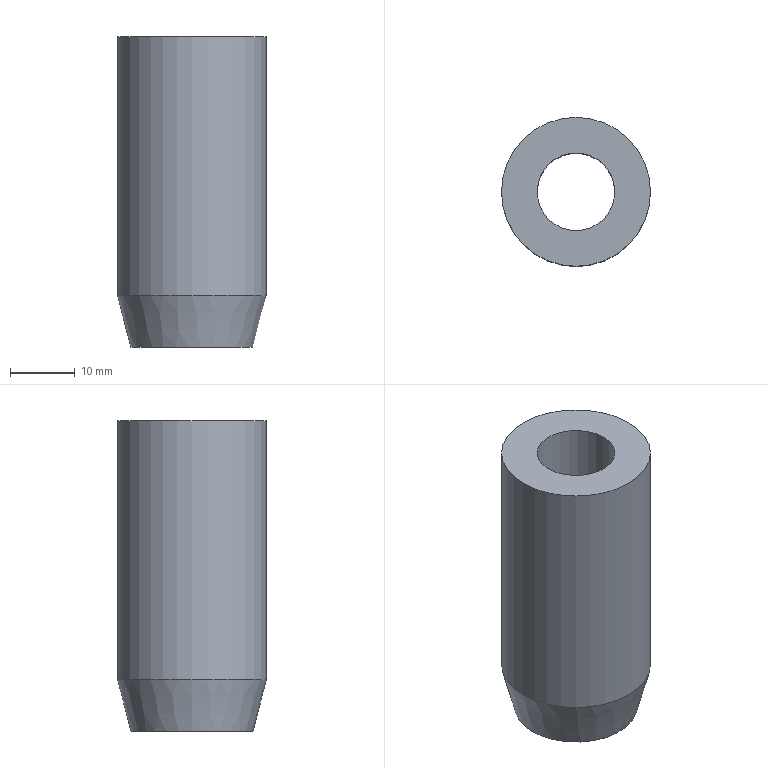Part | NX | features solid 2 | 1 solid | 5 faces | box 23 x 23 x 48 mm | volume 13952 mm3 | plane 2 | cylinder 2 | cone 1 | commonest cylinder face diameters 12 x1 23 x1
STEP:
#1=CARTESIAN_POINT('',(123.5,-300.,315.));
#2=VERTEX_POINT('',#1);
#3=CARTESIAN_POINT('',(135.,-300.,315.));
#4=DIRECTION('',(0.,0.,-1.));
#5=DIRECTION('',(-1.,0.,0.));
#6=AXIS2_PLACEMENT_3D('',#3,#4,#5);
#7=CIRCLE('',#6,11.5);
#8=EDGE_CURVE('',#2,#2,#7,.T.);
#9=ORIENTED_EDGE('',*,*,#8,.F.);
#10=EDGE_LOOP('',(#9));
#11=FACE_BOUND('',#10,.T.);
#12=CARTESIAN_POINT('',(129.,-300.,315.));
#13=VERTEX_POINT('',#12);
#14=CARTESIAN_POINT('',(135.,-300.,315.));
#15=DIRECTION('',(0.,0.,-1.));
#16=DIRECTION('',(-1.,0.,0.));
#17=AXIS2_PLACEMENT_3D('',#14,#15,#16);
#18=CIRCLE('',#17,6.);
#19=EDGE_CURVE('',#13,#13,#18,.T.);
#20=ORIENTED_EDGE('',*,*,#19,.T.);
#21=EDGE_LOOP('',(#20));
#22=FACE_BOUND('',#21,.T.);
#23=CARTESIAN_POINT('',(141.,-300.,315.));
#24=DIRECTION('',(0.,0.,-1.));
#25=DIRECTION('',(-1.,0.,0.));
#26=AXIS2_PLACEMENT_3D('',#23,#24,#25);
#27=PLANE('',#26);
#28=ADVANCED_FACE('',(#11,#22),#27,.F.);
#29=CARTESIAN_POINT('',(123.5,-300.,275.));
#30=VERTEX_POINT('',#29);
#31=CARTESIAN_POINT('',(135.,-300.,275.));
#32=DIRECTION('',(0.,0.,-1.));
#33=DIRECTION('',(-1.,0.,0.));
#34=AXIS2_PLACEMENT_3D('',#31,#32,#33);
#35=CIRCLE('',#34,11.5);
#36=EDGE_CURVE('',#30,#30,#35,.T.);
#37=ORIENTED_EDGE('',*,*,#36,.F.);
#38=EDGE_LOOP('',(#37));
#39=FACE_BOUND('',#38,.T.);
#40=ORIENTED_EDGE('',*,*,#8,.T.);
#41=EDGE_LOOP('',(#40));
#42=FACE_BOUND('',#41,.T.);
#43=CARTESIAN_POINT('',(135.,-300.,320.));
#44=DIRECTION('',(0.,0.,-1.));
#45=DIRECTION('',(-1.,0.,0.));
#46=AXIS2_PLACEMENT_3D('',#43,#44,#45);
#47=CYLINDRICAL_SURFACE('',#46,11.5);
#48=ADVANCED_FACE('',(#39,#42),#47,.T.);
#49=CARTESIAN_POINT('',(125.571,-300.,267.));
#50=VERTEX_POINT('',#49);
#51=CARTESIAN_POINT('',(135.,-300.,267.));
#52=DIRECTION('',(0.,0.,-1.));
#53=DIRECTION('',(-1.,0.,0.));
#54=AXIS2_PLACEMENT_3D('',#51,#52,#53);
#55=CIRCLE('',#54,9.429);
#56=EDGE_CURVE('',#50,#50,#55,.T.);
#57=ORIENTED_EDGE('',*,*,#56,.F.);
#58=EDGE_LOOP('',(#57));
#59=FACE_BOUND('',#58,.T.);
#60=ORIENTED_EDGE('',*,*,#36,.T.);
#61=EDGE_LOOP('',(#60));
#62=FACE_BOUND('',#61,.T.);
#63=CARTESIAN_POINT('',(135.,-300.,275.));
#64=DIRECTION('',(0.,0.,1.));
#65=DIRECTION('',(1.,0.,0.));
#66=AXIS2_PLACEMENT_3D('',#63,#64,#65);
#67=CONICAL_SURFACE('',#66,11.5,0.2533);
#68=ADVANCED_FACE('',(#59,#62),#67,.T.);
#69=CARTESIAN_POINT('',(129.,-300.,267.));
#70=VERTEX_POINT('',#69);
#71=CARTESIAN_POINT('',(135.,-300.,267.));
#72=DIRECTION('',(0.,0.,-1.));
#73=DIRECTION('',(-1.,0.,0.));
#74=AXIS2_PLACEMENT_3D('',#71,#72,#73);
#75=CIRCLE('',#74,6.);
#76=EDGE_CURVE('',#70,#70,#75,.T.);
#77=ORIENTED_EDGE('',*,*,#76,.F.);
#78=EDGE_LOOP('',(#77));
#79=FACE_BOUND('',#78,.T.);
#80=ORIENTED_EDGE('',*,*,#56,.T.);
#81=EDGE_LOOP('',(#80));
#82=FACE_BOUND('',#81,.T.);
#83=CARTESIAN_POINT('',(144.429,-300.,267.));
#84=DIRECTION('',(0.,0.,1.));
#85=DIRECTION('',(1.,0.,0.));
#86=AXIS2_PLACEMENT_3D('',#83,#84,#85);
#87=PLANE('',#86);
#88=ADVANCED_FACE('',(#79,#82),#87,.F.);
#89=ORIENTED_EDGE('',*,*,#19,.F.);
#90=EDGE_LOOP('',(#89));
#91=FACE_BOUND('',#90,.T.);
#92=ORIENTED_EDGE('',*,*,#76,.T.);
#93=EDGE_LOOP('',(#92));
#94=FACE_BOUND('',#93,.T.);
#95=CARTESIAN_POINT('',(135.,-300.,320.));
#96=DIRECTION('',(0.,0.,-1.));
#97=DIRECTION('',(-1.,0.,0.));
#98=AXIS2_PLACEMENT_3D('',#95,#96,#97);
#99=CYLINDRICAL_SURFACE('',#98,6.);
#100=ADVANCED_FACE('',(#91,#94),#99,.F.);
#101=CLOSED_SHELL('',(#28,#48,#68,#88,#100));
#102=MANIFOLD_SOLID_BREP('',#101);
#103=(LENGTH_UNIT()NAMED_UNIT(*)SI_UNIT(.MILLI.,.METRE.));
#104=UNCERTAINTY_MEASURE_WITH_UNIT(LENGTH_MEASURE(0.00001),#103,'','');
#105=(NAMED_UNIT(*)PLANE_ANGLE_UNIT()SI_UNIT($,.RADIAN.));
#106=(NAMED_UNIT(*)SI_UNIT($,.STERADIAN.)SOLID_ANGLE_UNIT());
#107=(GEOMETRIC_REPRESENTATION_CONTEXT(3)GLOBAL_UNCERTAINTY_ASSIGNED_CONTEXT((#104))GLOBAL_UNIT_ASSIGNED_CONTEXT((#103,#105,#106))REPRESENTATION_CONTEXT('',''));
#108=ADVANCED_BREP_SHAPE_REPRESENTATION('',(#102),#107);